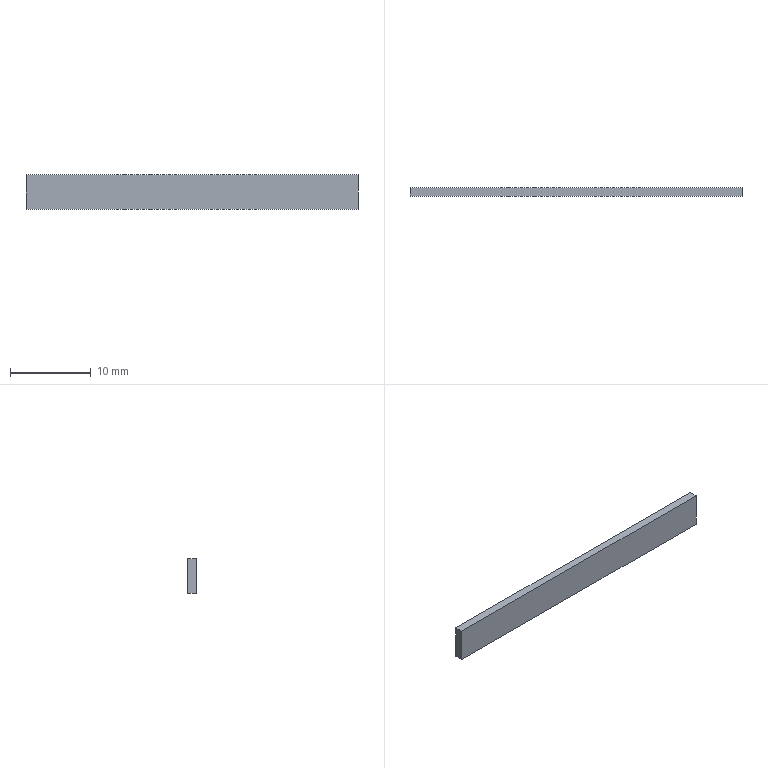Part | SolidWorks | features Extrusion 1 | 1 solid | 6 faces | box 41 x 1 x 4.3 mm | volume 176.3 mm3 | plane 6
STEP:
#1=CARTESIAN_POINT('',(0.,0.,-2.15));
#2=VERTEX_POINT('',#1);
#3=CARTESIAN_POINT('',(0.,0.,2.15));
#4=VERTEX_POINT('',#3);
#5=CARTESIAN_POINT('',(0.,0.,-2.15));
#6=DIRECTION('',(0.,0.,1.));
#7=VECTOR('',#6,1000.);
#8=LINE('',#5,#7);
#9=EDGE_CURVE('',#2,#4,#8,.T.);
#10=ORIENTED_EDGE('',*,*,#9,.T.);
#11=CARTESIAN_POINT('',(0.,1.,2.15));
#12=VERTEX_POINT('',#11);
#13=CARTESIAN_POINT('',(0.,1.,2.15));
#14=DIRECTION('',(0.,-1.,0.));
#15=VECTOR('',#14,1000.);
#16=LINE('',#13,#15);
#17=EDGE_CURVE('',#12,#4,#16,.T.);
#18=ORIENTED_EDGE('',*,*,#17,.F.);
#19=CARTESIAN_POINT('',(0.,1.,-2.15));
#20=VERTEX_POINT('',#19);
#21=CARTESIAN_POINT('',(0.,1.,-2.15));
#22=DIRECTION('',(0.,0.,1.));
#23=VECTOR('',#22,1000.);
#24=LINE('',#21,#23);
#25=EDGE_CURVE('',#20,#12,#24,.T.);
#26=ORIENTED_EDGE('',*,*,#25,.F.);
#27=CARTESIAN_POINT('',(0.,1.,-2.15));
#28=DIRECTION('',(0.,-1.,0.));
#29=VECTOR('',#28,1000.);
#30=LINE('',#27,#29);
#31=EDGE_CURVE('',#20,#2,#30,.T.);
#32=ORIENTED_EDGE('',*,*,#31,.T.);
#33=EDGE_LOOP('',(#10,#18,#26,#32));
#34=FACE_OUTER_BOUND('',#33,.T.);
#35=CARTESIAN_POINT('',(0.,1.,-2.15));
#36=DIRECTION('',(1.,0.,0.));
#37=DIRECTION('',(0.,0.,-1.));
#38=AXIS2_PLACEMENT_3D('',#35,#36,#37);
#39=PLANE('',#38);
#40=ADVANCED_FACE('',(#34),#39,.F.);
#41=CARTESIAN_POINT('',(41.,0.,2.15));
#42=VERTEX_POINT('',#41);
#43=CARTESIAN_POINT('',(0.,0.,2.15));
#44=DIRECTION('',(1.,0.,0.));
#45=VECTOR('',#44,1000.);
#46=LINE('',#43,#45);
#47=EDGE_CURVE('',#4,#42,#46,.T.);
#48=ORIENTED_EDGE('',*,*,#47,.T.);
#49=CARTESIAN_POINT('',(41.,1.,2.15));
#50=VERTEX_POINT('',#49);
#51=CARTESIAN_POINT('',(41.,1.,2.15));
#52=DIRECTION('',(0.,-1.,0.));
#53=VECTOR('',#52,1000.);
#54=LINE('',#51,#53);
#55=EDGE_CURVE('',#50,#42,#54,.T.);
#56=ORIENTED_EDGE('',*,*,#55,.F.);
#57=CARTESIAN_POINT('',(0.,1.,2.15));
#58=DIRECTION('',(1.,0.,0.));
#59=VECTOR('',#58,1000.);
#60=LINE('',#57,#59);
#61=EDGE_CURVE('',#12,#50,#60,.T.);
#62=ORIENTED_EDGE('',*,*,#61,.F.);
#63=ORIENTED_EDGE('',*,*,#17,.T.);
#64=EDGE_LOOP('',(#48,#56,#62,#63));
#65=FACE_OUTER_BOUND('',#64,.T.);
#66=CARTESIAN_POINT('',(0.,1.,2.15));
#67=DIRECTION('',(0.,0.,-1.));
#68=DIRECTION('',(-1.,0.,0.));
#69=AXIS2_PLACEMENT_3D('',#66,#67,#68);
#70=PLANE('',#69);
#71=ADVANCED_FACE('',(#65),#70,.F.);
#72=CARTESIAN_POINT('',(41.,0.,-2.15));
#73=VERTEX_POINT('',#72);
#74=CARTESIAN_POINT('',(41.,0.,-2.15));
#75=DIRECTION('',(0.,0.,-1.));
#76=VECTOR('',#75,1000.);
#77=LINE('',#74,#76);
#78=EDGE_CURVE('',#42,#73,#77,.T.);
#79=ORIENTED_EDGE('',*,*,#78,.T.);
#80=CARTESIAN_POINT('',(41.,1.,-2.15));
#81=VERTEX_POINT('',#80);
#82=CARTESIAN_POINT('',(41.,1.,-2.15));
#83=DIRECTION('',(0.,-1.,0.));
#84=VECTOR('',#83,1000.);
#85=LINE('',#82,#84);
#86=EDGE_CURVE('',#81,#73,#85,.T.);
#87=ORIENTED_EDGE('',*,*,#86,.F.);
#88=CARTESIAN_POINT('',(41.,1.,-2.15));
#89=DIRECTION('',(0.,0.,-1.));
#90=VECTOR('',#89,1000.);
#91=LINE('',#88,#90);
#92=EDGE_CURVE('',#50,#81,#91,.T.);
#93=ORIENTED_EDGE('',*,*,#92,.F.);
#94=ORIENTED_EDGE('',*,*,#55,.T.);
#95=EDGE_LOOP('',(#79,#87,#93,#94));
#96=FACE_OUTER_BOUND('',#95,.T.);
#97=CARTESIAN_POINT('',(41.,1.,-2.15));
#98=DIRECTION('',(-1.,0.,0.));
#99=DIRECTION('',(0.,0.,1.));
#100=AXIS2_PLACEMENT_3D('',#97,#98,#99);
#101=PLANE('',#100);
#102=ADVANCED_FACE('',(#96),#101,.F.);
#103=CARTESIAN_POINT('',(0.,0.,-2.15));
#104=DIRECTION('',(-1.,0.,0.));
#105=VECTOR('',#104,1000.);
#106=LINE('',#103,#105);
#107=EDGE_CURVE('',#73,#2,#106,.T.);
#108=ORIENTED_EDGE('',*,*,#107,.T.);
#109=ORIENTED_EDGE('',*,*,#31,.F.);
#110=CARTESIAN_POINT('',(0.,1.,-2.15));
#111=DIRECTION('',(-1.,0.,0.));
#112=VECTOR('',#111,1000.);
#113=LINE('',#110,#112);
#114=EDGE_CURVE('',#81,#20,#113,.T.);
#115=ORIENTED_EDGE('',*,*,#114,.F.);
#116=ORIENTED_EDGE('',*,*,#86,.T.);
#117=EDGE_LOOP('',(#108,#109,#115,#116));
#118=FACE_OUTER_BOUND('',#117,.T.);
#119=CARTESIAN_POINT('',(0.,1.,-2.15));
#120=DIRECTION('',(0.,0.,1.));
#121=DIRECTION('',(1.,0.,0.));
#122=AXIS2_PLACEMENT_3D('',#119,#120,#121);
#123=PLANE('',#122);
#124=ADVANCED_FACE('',(#118),#123,.F.);
#125=ORIENTED_EDGE('',*,*,#25,.T.);
#126=ORIENTED_EDGE('',*,*,#61,.T.);
#127=ORIENTED_EDGE('',*,*,#92,.T.);
#128=ORIENTED_EDGE('',*,*,#114,.T.);
#129=EDGE_LOOP('',(#125,#126,#127,#128));
#130=FACE_OUTER_BOUND('',#129,.T.);
#131=CARTESIAN_POINT('',(0.,1.,0.));
#132=DIRECTION('',(0.,1.,0.));
#133=DIRECTION('',(0.,0.,1.));
#134=AXIS2_PLACEMENT_3D('',#131,#132,#133);
#135=PLANE('',#134);
#136=ADVANCED_FACE('',(#130),#135,.T.);
#137=ORIENTED_EDGE('',*,*,#9,.F.);
#138=ORIENTED_EDGE('',*,*,#107,.F.);
#139=ORIENTED_EDGE('',*,*,#78,.F.);
#140=ORIENTED_EDGE('',*,*,#47,.F.);
#141=EDGE_LOOP('',(#137,#138,#139,#140));
#142=FACE_OUTER_BOUND('',#141,.T.);
#143=CARTESIAN_POINT('',(0.,0.,0.));
#144=DIRECTION('',(0.,1.,0.));
#145=DIRECTION('',(0.,0.,1.));
#146=AXIS2_PLACEMENT_3D('',#143,#144,#145);
#147=PLANE('',#146);
#148=ADVANCED_FACE('',(#142),#147,.F.);
#149=CLOSED_SHELL('',(#40,#71,#102,#124,#136,#148));
#150=MANIFOLD_SOLID_BREP('',#149);
#151=CARTESIAN_POINT('',(0.,0.,0.));
#152=DIRECTION('',(0.,0.,1.));
#153=DIRECTION('',(1.,0.,0.));
#154=AXIS2_PLACEMENT_3D('',#151,#152,#153);
#155=(LENGTH_UNIT()NAMED_UNIT(*)SI_UNIT(.MILLI.,.METRE.));
#156=UNCERTAINTY_MEASURE_WITH_UNIT(LENGTH_MEASURE(0.00001),#155,'','');
#157=(NAMED_UNIT(*)PLANE_ANGLE_UNIT()SI_UNIT($,.RADIAN.));
#158=(NAMED_UNIT(*)SI_UNIT($,.STERADIAN.)SOLID_ANGLE_UNIT());
#159=(GEOMETRIC_REPRESENTATION_CONTEXT(3)GLOBAL_UNCERTAINTY_ASSIGNED_CONTEXT((#156))GLOBAL_UNIT_ASSIGNED_CONTEXT((#155,#157,#158))REPRESENTATION_CONTEXT('',''));
#160=ADVANCED_BREP_SHAPE_REPRESENTATION('',(#150,#154),#159);